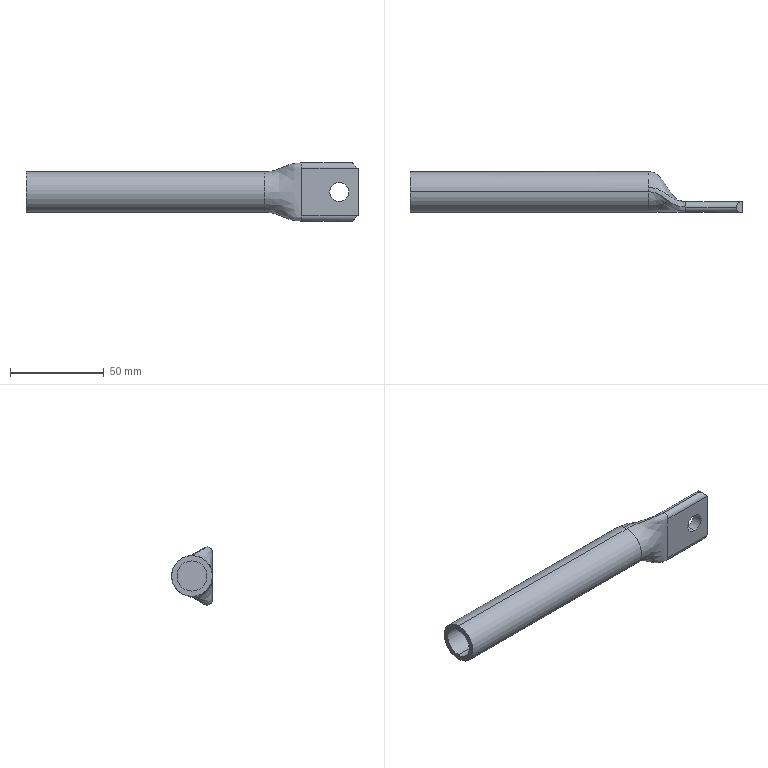Part | SolidWorks | features ICE 3, Chamfer 2, Blend 1, ExtruThin 1 | 1 solid | 28 faces | box 177 x 21.701 x 31 mm | volume 30996 mm3 | plane 15 | cylinder 10 | spline 3 | commonest cylinder face diameters 5.58 x4 10 x2 16.1 x2 21.7 x2
STEP:
#1=CARTESIAN_POINT('',(167.,-10.85,5.));
#2=VERTEX_POINT('',#1);
#3=CARTESIAN_POINT('',(167.,-10.85,-5.));
#4=VERTEX_POINT('',#3);
#5=CARTESIAN_POINT('',(167.,-10.85,0.));
#6=DIRECTION('',(0.,-1.,0.));
#7=DIRECTION('',(0.,0.,1.));
#8=AXIS2_PLACEMENT_3D('',#5,#6,#7);
#9=CIRCLE('',#8,5.);
#10=EDGE_CURVE('',#2,#4,#9,.T.);
#11=ORIENTED_EDGE('',*,*,#10,.T.);
#12=CARTESIAN_POINT('',(167.,-5.25,-5.));
#13=VERTEX_POINT('',#12);
#14=CARTESIAN_POINT('',(167.,-11.797,-5.));
#15=DIRECTION('',(0.,1.,0.));
#16=VECTOR('',#15,1000.);
#17=LINE('',#14,#16);
#18=EDGE_CURVE('',#4,#13,#17,.T.);
#19=ORIENTED_EDGE('',*,*,#18,.T.);
#20=CARTESIAN_POINT('',(167.,-5.25,5.));
#21=VERTEX_POINT('',#20);
#22=CARTESIAN_POINT('',(167.,-5.25,0.));
#23=DIRECTION('',(0.,1.,0.));
#24=DIRECTION('',(0.,0.,1.));
#25=AXIS2_PLACEMENT_3D('',#22,#23,#24);
#26=CIRCLE('',#25,5.);
#27=EDGE_CURVE('',#13,#21,#26,.T.);
#28=ORIENTED_EDGE('',*,*,#27,.T.);
#29=CARTESIAN_POINT('',(167.,-11.797,5.));
#30=DIRECTION('',(0.,1.,0.));
#31=VECTOR('',#30,1000.);
#32=LINE('',#29,#31);
#33=EDGE_CURVE('',#2,#21,#32,.T.);
#34=ORIENTED_EDGE('',*,*,#33,.F.);
#35=EDGE_LOOP('',(#11,#19,#28,#34));
#36=FACE_OUTER_BOUND('',#35,.T.);
#37=CARTESIAN_POINT('',(167.,-11.797,0.));
#38=DIRECTION('',(0.,1.,0.));
#39=DIRECTION('',(0.,0.,1.));
#40=AXIS2_PLACEMENT_3D('',#37,#38,#39);
#41=CYLINDRICAL_SURFACE('',#40,5.);
#42=ADVANCED_FACE('',(#36),#41,.F.);
#43=CARTESIAN_POINT('',(127.,0.,8.05));
#44=VERTEX_POINT('',#43);
#45=CARTESIAN_POINT('',(127.,0.,-8.05));
#46=VERTEX_POINT('',#45);
#47=CARTESIAN_POINT('',(127.,0.,0.));
#48=DIRECTION('',(1.,0.,0.));
#49=DIRECTION('',(0.,0.,-1.));
#50=AXIS2_PLACEMENT_3D('',#47,#48,#49);
#51=CIRCLE('',#50,8.05);
#52=EDGE_CURVE('',#44,#46,#51,.T.);
#53=ORIENTED_EDGE('',*,*,#52,.T.);
#54=CARTESIAN_POINT('',(0.,0.,-8.05));
#55=VERTEX_POINT('',#54);
#56=CARTESIAN_POINT('',(127.,0.,-8.05));
#57=DIRECTION('',(-1.,0.,0.));
#58=VECTOR('',#57,1000.);
#59=LINE('',#56,#58);
#60=EDGE_CURVE('',#46,#55,#59,.T.);
#61=ORIENTED_EDGE('',*,*,#60,.T.);
#62=CARTESIAN_POINT('',(0.,0.,8.05));
#63=VERTEX_POINT('',#62);
#64=CARTESIAN_POINT('',(0.,0.,0.));
#65=DIRECTION('',(1.,0.,0.));
#66=DIRECTION('',(0.,0.,-1.));
#67=AXIS2_PLACEMENT_3D('',#64,#65,#66);
#68=CIRCLE('',#67,8.05);
#69=EDGE_CURVE('',#63,#55,#68,.T.);
#70=ORIENTED_EDGE('',*,*,#69,.F.);
#71=CARTESIAN_POINT('',(127.,0.,8.05));
#72=DIRECTION('',(-1.,0.,0.));
#73=VECTOR('',#72,1000.);
#74=LINE('',#71,#73);
#75=EDGE_CURVE('',#44,#63,#74,.T.);
#76=ORIENTED_EDGE('',*,*,#75,.F.);
#77=EDGE_LOOP('',(#53,#61,#70,#76));
#78=FACE_OUTER_BOUND('',#77,.T.);
#79=CARTESIAN_POINT('',(127.,0.,0.));
#80=DIRECTION('',(-1.,0.,0.));
#81=DIRECTION('',(0.,0.,1.));
#82=AXIS2_PLACEMENT_3D('',#79,#80,#81);
#83=CYLINDRICAL_SURFACE('',#82,8.05);
#84=ADVANCED_FACE('',(#78),#83,.F.);
#85=CARTESIAN_POINT('',(127.,0.00175,-10.85));
#86=VERTEX_POINT('',#85);
#87=CARTESIAN_POINT('',(127.,2.334,10.597));
#88=VERTEX_POINT('',#87);
#89=CARTESIAN_POINT('',(127.,0.00175,-10.85));
#90=CARTESIAN_POINT('',(127.,0.3537,-10.85));
#91=CARTESIAN_POINT('',(127.,0.5767,-10.839));
#92=CARTESIAN_POINT('',(127.,0.7699,-10.825));
#93=CARTESIAN_POINT('',(127.,1.177,-10.792));
#94=CARTESIAN_POINT('',(127.,1.582,-10.736));
#95=CARTESIAN_POINT('',(127.,1.774,-10.708));
#96=CARTESIAN_POINT('',(127.,1.994,-10.671));
#97=CARTESIAN_POINT('',(127.,2.677,-10.52));
#98=CARTESIAN_POINT('',(127.,3.018,-10.431));
#99=CARTESIAN_POINT('',(127.,3.357,-10.326));
#100=CARTESIAN_POINT('',(127.,6.037,-9.379));
#101=CARTESIAN_POINT('',(127.,8.44,-7.529));
#102=CARTESIAN_POINT('',(127.,10.034,-5.273));
#103=CARTESIAN_POINT('',(127.,11.771,0.3481));
#104=CARTESIAN_POINT('',(127.,9.812,5.985));
#105=CARTESIAN_POINT('',(127.,7.737,8.454));
#106=CARTESIAN_POINT('',(127.,5.094,9.988));
#107=CARTESIAN_POINT('',(127.,2.334,10.597));
#108=B_SPLINE_CURVE_WITH_KNOTS('',5,(#89,#90,#91,#92,#93,#94,#95,#96,#97,#98,#99,#100,#101,#102,#103,#104,#105,#106,#107),.UNSPECIFIED.,.F.,.F.,(6,3,4,3,3,6),(0.,0.05525,0.1105,0.1661,0.5552,1.),.UNSPECIFIED.);
#109=EDGE_CURVE('',#86,#88,#108,.T.);
#110=ORIENTED_EDGE('',*,*,#109,.F.);
#111=CARTESIAN_POINT('',(0.,0.,-10.85));
#112=VERTEX_POINT('',#111);
#113=CARTESIAN_POINT('',(127.,0.,-10.85));
#114=DIRECTION('',(-1.,0.,0.));
#115=VECTOR('',#114,1000.);
#116=LINE('',#113,#115);
#117=EDGE_CURVE('',#86,#112,#116,.T.);
#118=ORIENTED_EDGE('',*,*,#117,.T.);
#119=CARTESIAN_POINT('',(0.,0.,10.85));
#120=VERTEX_POINT('',#119);
#121=CARTESIAN_POINT('',(0.,0.,0.));
#122=DIRECTION('',(1.,0.,0.));
#123=DIRECTION('',(0.,0.,-1.));
#124=AXIS2_PLACEMENT_3D('',#121,#122,#123);
#125=CIRCLE('',#124,10.85);
#126=EDGE_CURVE('',#112,#120,#125,.T.);
#127=ORIENTED_EDGE('',*,*,#126,.T.);
#128=CARTESIAN_POINT('',(127.,0.000003204,10.85));
#129=VERTEX_POINT('',#128);
#130=CARTESIAN_POINT('',(127.,0.,10.85));
#131=DIRECTION('',(-1.,0.,0.));
#132=VECTOR('',#131,1000.);
#133=LINE('',#130,#132);
#134=EDGE_CURVE('',#129,#120,#133,.T.);
#135=ORIENTED_EDGE('',*,*,#134,.F.);
#136=CARTESIAN_POINT('',(127.,0.,0.));
#137=DIRECTION('',(1.,0.,0.));
#138=DIRECTION('',(0.,0.,-1.));
#139=AXIS2_PLACEMENT_3D('',#136,#137,#138);
#140=CIRCLE('',#139,10.85);
#141=EDGE_CURVE('',#88,#129,#140,.T.);
#142=ORIENTED_EDGE('',*,*,#141,.F.);
#143=EDGE_LOOP('',(#110,#118,#127,#135,#142));
#144=FACE_OUTER_BOUND('',#143,.T.);
#145=CARTESIAN_POINT('',(127.,0.,0.));
#146=DIRECTION('',(-1.,0.,0.));
#147=DIRECTION('',(0.,0.,1.));
#148=AXIS2_PLACEMENT_3D('',#145,#146,#147);
#149=CYLINDRICAL_SURFACE('',#148,10.85);
#150=ADVANCED_FACE('',(#144),#149,.T.);
#151=CARTESIAN_POINT('',(177.,-8.1,12.5));
#152=VERTEX_POINT('',#151);
#153=CARTESIAN_POINT('',(177.,-8.1,-12.5));
#154=VERTEX_POINT('',#153);
#155=CARTESIAN_POINT('',(177.,-8.1,-12.5));
#156=DIRECTION('',(0.,0.,-1.));
#157=VECTOR('',#156,1000.);
#158=LINE('',#155,#157);
#159=EDGE_CURVE('',#152,#154,#158,.T.);
#160=ORIENTED_EDGE('',*,*,#159,.F.);
#161=CARTESIAN_POINT('',(177.,-10.85,12.5));
#162=VERTEX_POINT('',#161);
#163=CARTESIAN_POINT('',(177.,-8.06,12.5));
#164=DIRECTION('',(0.,-1.,0.));
#165=VECTOR('',#164,1000.);
#166=LINE('',#163,#165);
#167=EDGE_CURVE('',#152,#162,#166,.T.);
#168=ORIENTED_EDGE('',*,*,#167,.T.);
#169=CARTESIAN_POINT('',(177.,-10.85,-12.5));
#170=VERTEX_POINT('',#169);
#171=CARTESIAN_POINT('',(177.,-10.85,12.71));
#172=DIRECTION('',(0.,0.,-1.));
#173=VECTOR('',#172,1000.);
#174=LINE('',#171,#173);
#175=EDGE_CURVE('',#162,#170,#174,.T.);
#176=ORIENTED_EDGE('',*,*,#175,.T.);
#177=CARTESIAN_POINT('',(177.,-8.04,-12.5));
#178=DIRECTION('',(0.,1.,0.));
#179=VECTOR('',#178,1000.);
#180=LINE('',#177,#179);
#181=EDGE_CURVE('',#170,#154,#180,.T.);
#182=ORIENTED_EDGE('',*,*,#181,.T.);
#183=EDGE_LOOP('',(#160,#168,#176,#182));
#184=FACE_OUTER_BOUND('',#183,.T.);
#185=CARTESIAN_POINT('',(177.,-8.06,-12.71));
#186=DIRECTION('',(1.,0.,0.));
#187=DIRECTION('',(0.,0.,-1.));
#188=AXIS2_PLACEMENT_3D('',#185,#186,#187);
#189=PLANE('',#188);
#190=ADVANCED_FACE('',(#184),#189,.T.);
#191=CARTESIAN_POINT('',(0.,0.,0.));
#192=DIRECTION('',(1.,0.,0.));
#193=DIRECTION('',(0.,0.,-1.));
#194=AXIS2_PLACEMENT_3D('',#191,#192,#193);
#195=CIRCLE('',#194,10.85);
#196=EDGE_CURVE('',#120,#112,#195,.T.);
#197=ORIENTED_EDGE('',*,*,#196,.F.);
#198=ORIENTED_EDGE('',*,*,#126,.F.);
#199=EDGE_LOOP('',(#197,#198));
#200=FACE_OUTER_BOUND('',#199,.T.);
#201=ORIENTED_EDGE('',*,*,#69,.T.);
#202=CARTESIAN_POINT('',(0.,0.,0.));
#203=DIRECTION('',(1.,0.,0.));
#204=DIRECTION('',(0.,0.,-1.));
#205=AXIS2_PLACEMENT_3D('',#202,#203,#204);
#206=CIRCLE('',#205,8.05);
#207=EDGE_CURVE('',#55,#63,#206,.T.);
#208=ORIENTED_EDGE('',*,*,#207,.T.);
#209=EDGE_LOOP('',(#201,#208));
#210=FACE_BOUND('',#209,.T.);
#211=CARTESIAN_POINT('',(0.,0.,0.));
#212=DIRECTION('',(1.,0.,0.));
#213=DIRECTION('',(0.,0.,-1.));
#214=AXIS2_PLACEMENT_3D('',#211,#212,#213);
#215=PLANE('',#214);
#216=ADVANCED_FACE('',(#200,#210),#215,.F.);
#217=ORIENTED_EDGE('',*,*,#117,.F.);
#218=CARTESIAN_POINT('',(127.,0.,0.));
#219=DIRECTION('',(1.,0.,0.));
#220=DIRECTION('',(0.,0.,-1.));
#221=AXIS2_PLACEMENT_3D('',#218,#219,#220);
#222=CIRCLE('',#221,10.85);
#223=EDGE_CURVE('',#129,#86,#222,.T.);
#224=ORIENTED_EDGE('',*,*,#223,.F.);
#225=ORIENTED_EDGE('',*,*,#134,.T.);
#226=ORIENTED_EDGE('',*,*,#196,.T.);
#227=EDGE_LOOP('',(#217,#224,#225,#226));
#228=FACE_OUTER_BOUND('',#227,.T.);
#229=CARTESIAN_POINT('',(127.,0.,0.));
#230=DIRECTION('',(-1.,0.,0.));
#231=DIRECTION('',(0.,0.,1.));
#232=AXIS2_PLACEMENT_3D('',#229,#230,#231);
#233=CYLINDRICAL_SURFACE('',#232,10.85);
#234=ADVANCED_FACE('',(#228),#233,.T.);
#235=ORIENTED_EDGE('',*,*,#60,.F.);
#236=CARTESIAN_POINT('',(127.,0.,0.));
#237=DIRECTION('',(1.,0.,0.));
#238=DIRECTION('',(0.,0.,-1.));
#239=AXIS2_PLACEMENT_3D('',#236,#237,#238);
#240=CIRCLE('',#239,8.05);
#241=EDGE_CURVE('',#46,#44,#240,.T.);
#242=ORIENTED_EDGE('',*,*,#241,.T.);
#243=ORIENTED_EDGE('',*,*,#75,.T.);
#244=ORIENTED_EDGE('',*,*,#207,.F.);
#245=EDGE_LOOP('',(#235,#242,#243,#244));
#246=FACE_OUTER_BOUND('',#245,.T.);
#247=CARTESIAN_POINT('',(127.,0.,0.));
#248=DIRECTION('',(-1.,0.,0.));
#249=DIRECTION('',(0.,0.,1.));
#250=AXIS2_PLACEMENT_3D('',#247,#248,#249);
#251=CYLINDRICAL_SURFACE('',#250,8.05);
#252=ADVANCED_FACE('',(#246),#251,.F.);
#253=ORIENTED_EDGE('',*,*,#52,.F.);
#254=ORIENTED_EDGE('',*,*,#241,.F.);
#255=EDGE_LOOP('',(#253,#254));
#256=FACE_OUTER_BOUND('',#255,.T.);
#257=CARTESIAN_POINT('',(127.,0.,0.));
#258=DIRECTION('',(1.,0.,0.));
#259=DIRECTION('',(0.,0.,-1.));
#260=AXIS2_PLACEMENT_3D('',#257,#258,#259);
#261=PLANE('',#260);
#262=ADVANCED_FACE('',(#256),#261,.F.);
#263=CARTESIAN_POINT('',(147.,-5.25,12.71));
#264=VERTEX_POINT('',#263);
#265=CARTESIAN_POINT('',(147.,-5.25,12.71));
#266=CARTESIAN_POINT('',(142.97,-5.25,12.71));
#267=CARTESIAN_POINT('',(138.94,-5.25,12.71));
#268=CARTESIAN_POINT('',(135.06,2.334,10.596));
#269=CARTESIAN_POINT('',(131.03,2.334,10.596));
#270=CARTESIAN_POINT('',(127.,2.334,10.597));
#271=B_SPLINE_CURVE_WITH_KNOTS('',5,(#265,#266,#267,#268,#269,#270),.UNSPECIFIED.,.F.,.F.,(6,6),(0.,1.),.UNSPECIFIED.);
#272=EDGE_CURVE('',#264,#88,#271,.T.);
#273=ORIENTED_EDGE('',*,*,#272,.F.);
#274=CARTESIAN_POINT('',(147.,-5.25,-12.71));
#275=VERTEX_POINT('',#274);
#276=CARTESIAN_POINT('',(147.,-5.25,12.71));
#277=DIRECTION('',(0.,0.,-1.));
#278=VECTOR('',#277,1000.);
#279=LINE('',#276,#278);
#280=EDGE_CURVE('',#264,#275,#279,.T.);
#281=ORIENTED_EDGE('',*,*,#280,.T.);
#282=CARTESIAN_POINT('',(147.,-8.054,-15.5));
#283=VERTEX_POINT('',#282);
#284=CARTESIAN_POINT('',(147.,-5.25,-12.71));
#285=CARTESIAN_POINT('',(147.,-5.25,-13.038));
#286=CARTESIAN_POINT('',(147.,-5.297,-13.412));
#287=CARTESIAN_POINT('',(147.,-5.413,-13.847));
#288=CARTESIAN_POINT('',(147.,-5.978,-14.779));
#289=CARTESIAN_POINT('',(147.,-6.91,-15.339));
#290=CARTESIAN_POINT('',(147.,-7.342,-15.453));
#291=CARTESIAN_POINT('',(147.,-7.714,-15.5));
#292=CARTESIAN_POINT('',(147.,-8.054,-15.5));
#293=B_SPLINE_CURVE_WITH_KNOTS('',5,(#284,#285,#286,#287,#288,#289,#290,#291,#292),.UNSPECIFIED.,.F.,.F.,(6,3,6),(0.8895,0.9448,1.),.UNSPECIFIED.);
#294=EDGE_CURVE('',#275,#283,#293,.T.);
#295=ORIENTED_EDGE('',*,*,#294,.T.);
#296=CARTESIAN_POINT('',(147.,-8.054,-15.5));
#297=CARTESIAN_POINT('',(142.959,-8.04,-15.5));
#298=CARTESIAN_POINT('',(138.918,-8.04,-15.5));
#299=CARTESIAN_POINT('',(135.082,0.007,-10.85));
#300=CARTESIAN_POINT('',(131.041,0.007,-10.85));
#301=CARTESIAN_POINT('',(127.,0.00175,-10.85));
#302=B_SPLINE_CURVE_WITH_KNOTS('',5,(#296,#297,#298,#299,#300,#301),.UNSPECIFIED.,.F.,.F.,(6,6),(0.,1.),.UNSPECIFIED.);
#303=EDGE_CURVE('',#283,#86,#302,.T.);
#304=ORIENTED_EDGE('',*,*,#303,.T.);
#305=ORIENTED_EDGE('',*,*,#109,.T.);
#306=EDGE_LOOP('',(#273,#281,#295,#304,#305));
#307=FACE_OUTER_BOUND('',#306,.T.);
#308=CARTESIAN_POINT('',(147.,-8.04,-15.5));
#309=CARTESIAN_POINT('',(142.959,-8.04,-15.5));
#310=CARTESIAN_POINT('',(138.918,-8.04,-15.5));
#311=CARTESIAN_POINT('',(135.082,0.007,-10.85));
#312=CARTESIAN_POINT('',(131.041,0.007,-10.85));
#313=CARTESIAN_POINT('',(127.,0.007,-10.85));
#314=CARTESIAN_POINT('',(147.,-7.714,-15.5));
#315=CARTESIAN_POINT('',(142.962,-7.714,-15.5));
#316=CARTESIAN_POINT('',(138.924,-7.714,-15.5));
#317=CARTESIAN_POINT('',(135.076,0.3537,-10.85));
#318=CARTESIAN_POINT('',(131.038,0.3537,-10.85));
#319=CARTESIAN_POINT('',(127.,0.3537,-10.85));
#320=CARTESIAN_POINT('',(147.,-7.342,-15.453));
#321=CARTESIAN_POINT('',(142.965,-7.342,-15.453));
#322=CARTESIAN_POINT('',(138.929,-7.342,-15.453));
#323=CARTESIAN_POINT('',(135.071,0.5767,-10.839));
#324=CARTESIAN_POINT('',(131.035,0.5767,-10.839));
#325=CARTESIAN_POINT('',(127.,0.5767,-10.839));
#326=CARTESIAN_POINT('',(147.,-6.91,-15.339));
#327=CARTESIAN_POINT('',(142.967,-6.91,-15.339));
#328=CARTESIAN_POINT('',(138.934,-6.91,-15.339));
#329=CARTESIAN_POINT('',(135.066,0.7699,-10.825));
#330=CARTESIAN_POINT('',(131.033,0.7699,-10.825));
#331=CARTESIAN_POINT('',(127.,0.7699,-10.825));
#332=CARTESIAN_POINT('',(147.,-5.978,-14.779));
#333=CARTESIAN_POINT('',(142.97,-5.978,-14.779));
#334=CARTESIAN_POINT('',(138.939,-5.978,-14.779));
#335=CARTESIAN_POINT('',(135.061,1.177,-10.792));
#336=CARTESIAN_POINT('',(131.03,1.177,-10.792));
#337=CARTESIAN_POINT('',(127.,1.177,-10.792));
#338=CARTESIAN_POINT('',(147.,-5.413,-13.847));
#339=CARTESIAN_POINT('',(142.968,-5.413,-13.847));
#340=CARTESIAN_POINT('',(138.936,-5.413,-13.847));
#341=CARTESIAN_POINT('',(135.064,1.582,-10.736));
#342=CARTESIAN_POINT('',(131.032,1.582,-10.736));
#343=CARTESIAN_POINT('',(127.,1.582,-10.736));
#344=CARTESIAN_POINT('',(147.,-5.297,-13.412));
#345=CARTESIAN_POINT('',(142.966,-5.297,-13.412));
#346=CARTESIAN_POINT('',(138.931,-5.297,-13.412));
#347=CARTESIAN_POINT('',(135.069,1.774,-10.708));
#348=CARTESIAN_POINT('',(131.034,1.774,-10.708));
#349=CARTESIAN_POINT('',(127.,1.774,-10.708));
#350=CARTESIAN_POINT('',(147.,-5.25,-13.038));
#351=CARTESIAN_POINT('',(142.962,-5.25,-13.038));
#352=CARTESIAN_POINT('',(138.924,-5.25,-13.038));
#353=CARTESIAN_POINT('',(135.076,1.994,-10.671));
#354=CARTESIAN_POINT('',(131.038,1.994,-10.671));
#355=CARTESIAN_POINT('',(127.,1.994,-10.671));
#356=CARTESIAN_POINT('',(147.,-5.25,-12.38));
#357=CARTESIAN_POINT('',(142.95,-5.25,-12.38));
#358=CARTESIAN_POINT('',(138.9,-5.25,-12.38));
#359=CARTESIAN_POINT('',(135.1,2.677,-10.52));
#360=CARTESIAN_POINT('',(131.05,2.677,-10.52));
#361=CARTESIAN_POINT('',(127.,2.677,-10.52));
#362=CARTESIAN_POINT('',(147.,-5.25,-12.052));
#363=CARTESIAN_POINT('',(142.942,-5.25,-12.052));
#364=CARTESIAN_POINT('',(138.884,-5.25,-12.052));
#365=CARTESIAN_POINT('',(135.116,3.018,-10.431));
#366=CARTESIAN_POINT('',(131.058,3.018,-10.431));
#367=CARTESIAN_POINT('',(127.,3.018,-10.431));
#368=CARTESIAN_POINT('',(147.,-5.25,-11.724));
#369=CARTESIAN_POINT('',(142.939,-5.25,-11.724));
#370=CARTESIAN_POINT('',(138.878,-5.25,-11.724));
#371=CARTESIAN_POINT('',(135.122,3.357,-10.326));
#372=CARTESIAN_POINT('',(131.061,3.357,-10.326));
#373=CARTESIAN_POINT('',(127.,3.357,-10.326));
#374=CARTESIAN_POINT('',(147.,-5.25,-9.115));
#375=CARTESIAN_POINT('',(142.897,-5.25,-9.115));
#376=CARTESIAN_POINT('',(138.794,-5.25,-9.115));
#377=CARTESIAN_POINT('',(135.206,6.037,-9.379));
#378=CARTESIAN_POINT('',(131.103,6.037,-9.379));
#379=CARTESIAN_POINT('',(127.,6.037,-9.379));
#380=CARTESIAN_POINT('',(147.,-5.25,-6.573));
#381=CARTESIAN_POINT('',(142.868,-5.25,-6.573));
#382=CARTESIAN_POINT('',(138.736,-5.25,-6.573));
#383=CARTESIAN_POINT('',(135.264,8.44,-7.529));
#384=CARTESIAN_POINT('',(131.132,8.44,-7.529));
#385=CARTESIAN_POINT('',(127.,8.44,-7.529));
#386=CARTESIAN_POINT('',(147.,-5.25,-4.381));
#387=CARTESIAN_POINT('',(142.852,-5.25,-4.381));
#388=CARTESIAN_POINT('',(138.704,-5.25,-4.381));
#389=CARTESIAN_POINT('',(135.296,10.034,-5.273));
#390=CARTESIAN_POINT('',(131.148,10.034,-5.273));
#391=CARTESIAN_POINT('',(127.,10.034,-5.273));
#392=CARTESIAN_POINT('',(147.,-5.25,0.2909));
#393=CARTESIAN_POINT('',(142.838,-5.25,0.2909));
#394=CARTESIAN_POINT('',(138.676,-5.25,0.2909));
#395=CARTESIAN_POINT('',(135.324,11.771,0.3481));
#396=CARTESIAN_POINT('',(131.162,11.771,0.3481));
#397=CARTESIAN_POINT('',(127.,11.771,0.3481));
#398=CARTESIAN_POINT('',(147.,-5.25,4.969));
#399=CARTESIAN_POINT('',(142.865,-5.25,4.969));
#400=CARTESIAN_POINT('',(138.729,-5.25,4.969));
#401=CARTESIAN_POINT('',(135.271,9.812,5.985));
#402=CARTESIAN_POINT('',(131.135,9.812,5.985));
#403=CARTESIAN_POINT('',(127.,9.812,5.985));
#404=CARTESIAN_POINT('',(147.,-5.25,7.487));
#405=CARTESIAN_POINT('',(142.89,-5.25,7.487));
#406=CARTESIAN_POINT('',(138.779,-5.25,7.487));
#407=CARTESIAN_POINT('',(135.221,7.737,8.454));
#408=CARTESIAN_POINT('',(131.11,7.737,8.454));
#409=CARTESIAN_POINT('',(127.,7.737,8.454));
#410=CARTESIAN_POINT('',(147.,-5.25,10.055));
#411=CARTESIAN_POINT('',(142.925,-5.25,10.055));
#412=CARTESIAN_POINT('',(138.85,-5.25,10.055));
#413=CARTESIAN_POINT('',(135.15,5.094,9.988));
#414=CARTESIAN_POINT('',(131.075,5.094,9.988));
#415=CARTESIAN_POINT('',(127.,5.094,9.988));
#416=CARTESIAN_POINT('',(147.,-5.25,12.71));
#417=CARTESIAN_POINT('',(142.97,-5.25,12.71));
#418=CARTESIAN_POINT('',(138.94,-5.25,12.71));
#419=CARTESIAN_POINT('',(135.06,2.334,10.596));
#420=CARTESIAN_POINT('',(131.03,2.334,10.596));
#421=CARTESIAN_POINT('',(127.,2.334,10.596));
#422=B_SPLINE_SURFACE_WITH_KNOTS('',5,5,((#308,#309,#310,#311,#312,#313),(#314,#315,#316,#317,#318,#319),(#320,#321,#322,#323,#324,#325),(#326,#327,#328,#329,#330,#331),(#332,#333,#334,#335,#336,#337),(#338,#339,#340,#341,#342,#343),(#344,#345,#346,#347,#348,#349),(#350,#351,#352,#353,#354,#355),(#356,#357,#358,#359,#360,#361),(#362,#363,#364,#365,#366,#367),(#368,#369,#370,#371,#372,#373),(#374,#375,#376,#377,#378,#379),(#380,#381,#382,#383,#384,#385),(#386,#387,#388,#389,#390,#391),(#392,#393,#394,#395,#396,#397),(#398,#399,#400,#401,#402,#403),(#404,#405,#406,#407,#408,#409),(#410,#411,#412,#413,#414,#415),(#416,#417,#418,#419,#420,#421)),.UNSPECIFIED.,.F.,.F.,.F.,(6,3,4,3,3,6),(6,6),(0.,0.05525,0.1105,0.1661,0.5552,1.),(0.,1.),.UNSPECIFIED.);
#423=ADVANCED_FACE('',(#307),#422,.F.);
#424=ORIENTED_EDGE('',*,*,#272,.T.);
#425=ORIENTED_EDGE('',*,*,#141,.T.);
#426=CARTESIAN_POINT('',(147.,-8.046,15.5));
#427=VERTEX_POINT('',#426);
#428=CARTESIAN_POINT('',(147.,-8.046,15.5));
#429=CARTESIAN_POINT('',(142.959,-8.04,15.5));
#430=CARTESIAN_POINT('',(138.918,-8.04,15.5));
#431=CARTESIAN_POINT('',(135.082,0.007,10.85));
#432=CARTESIAN_POINT('',(131.041,0.007,10.85));
#433=CARTESIAN_POINT('',(127.,0.000003204,10.85));
#434=B_SPLINE_CURVE_WITH_KNOTS('',5,(#428,#429,#430,#431,#432,#433),.UNSPECIFIED.,.F.,.F.,(6,6),(0.,1.),.UNSPECIFIED.);
#435=EDGE_CURVE('',#427,#129,#434,.T.);
#436=ORIENTED_EDGE('',*,*,#435,.F.);
#437=CARTESIAN_POINT('',(147.,-8.04,12.71));
#438=DIRECTION('',(-1.,0.,0.));
#439=DIRECTION('',(0.,0.,1.));
#440=AXIS2_PLACEMENT_3D('',#437,#438,#439);
#441=CIRCLE('',#440,2.79);
#442=EDGE_CURVE('',#427,#264,#441,.T.);
#443=ORIENTED_EDGE('',*,*,#442,.T.);
#444=EDGE_LOOP('',(#424,#425,#436,#443));
#445=FACE_OUTER_BOUND('',#444,.T.);
#446=CARTESIAN_POINT('',(147.,-8.04,15.5));
#447=CARTESIAN_POINT('',(142.959,-8.04,15.5));
#448=CARTESIAN_POINT('',(138.918,-8.04,15.5));
#449=CARTESIAN_POINT('',(135.082,0.007,10.85));
#450=CARTESIAN_POINT('',(131.041,0.007,10.85));
#451=CARTESIAN_POINT('',(127.,0.007,10.85));
#452=CARTESIAN_POINT('',(147.,-7.116,15.5));
#453=CARTESIAN_POINT('',(142.959,-7.116,15.5));
#454=CARTESIAN_POINT('',(138.918,-7.116,15.5));
#455=CARTESIAN_POINT('',(135.082,0.4766,10.85));
#456=CARTESIAN_POINT('',(131.041,0.4766,10.85));
#457=CARTESIAN_POINT('',(127.,0.4766,10.85));
#458=CARTESIAN_POINT('',(147.,-6.279,15.125));
#459=CARTESIAN_POINT('',(142.961,-6.279,15.125));
#460=CARTESIAN_POINT('',(138.921,-6.279,15.125));
#461=CARTESIAN_POINT('',(135.079,0.9455,10.824));
#462=CARTESIAN_POINT('',(131.039,0.9455,10.824));
#463=CARTESIAN_POINT('',(127.,0.9455,10.824));
#464=CARTESIAN_POINT('',(147.,-5.625,14.471));
#465=CARTESIAN_POINT('',(142.963,-5.625,14.471));
#466=CARTESIAN_POINT('',(138.927,-5.625,14.471));
#467=CARTESIAN_POINT('',(135.073,1.412,10.773));
#468=CARTESIAN_POINT('',(131.037,1.412,10.773));
#469=CARTESIAN_POINT('',(127.,1.412,10.773));
#470=CARTESIAN_POINT('',(147.,-5.25,13.634));
#471=CARTESIAN_POINT('',(142.967,-5.25,13.634));
#472=CARTESIAN_POINT('',(138.934,-5.25,13.634));
#473=CARTESIAN_POINT('',(135.066,1.876,10.697));
#474=CARTESIAN_POINT('',(131.033,1.876,10.697));
#475=CARTESIAN_POINT('',(127.,1.876,10.697));
#476=CARTESIAN_POINT('',(147.,-5.25,12.71));
#477=CARTESIAN_POINT('',(142.97,-5.25,12.71));
#478=CARTESIAN_POINT('',(138.94,-5.25,12.71));
#479=CARTESIAN_POINT('',(135.06,2.334,10.596));
#480=CARTESIAN_POINT('',(131.03,2.334,10.596));
#481=CARTESIAN_POINT('',(127.,2.334,10.596));
#482=B_SPLINE_SURFACE_WITH_KNOTS('',5,5,((#446,#447,#448,#449,#450,#451),(#452,#453,#454,#455,#456,#457),(#458,#459,#460,#461,#462,#463),(#464,#465,#466,#467,#468,#469),(#470,#471,#472,#473,#474,#475),(#476,#477,#478,#479,#480,#481)),.UNSPECIFIED.,.F.,.F.,.F.,(6,6),(6,6),(0.,1.),(0.,1.),.UNSPECIFIED.);
#483=ADVANCED_FACE('',(#445),#482,.T.);
#484=ORIENTED_EDGE('',*,*,#303,.F.);
#485=CARTESIAN_POINT('',(147.,-10.85,-12.71));
#486=VERTEX_POINT('',#485);
#487=CARTESIAN_POINT('',(147.,-8.06,-12.71));
#488=DIRECTION('',(-1.,0.,0.));
#489=DIRECTION('',(0.,0.,1.));
#490=AXIS2_PLACEMENT_3D('',#487,#488,#489);
#491=CIRCLE('',#490,2.79);
#492=EDGE_CURVE('',#283,#486,#491,.T.);
#493=ORIENTED_EDGE('',*,*,#492,.T.);
#494=CARTESIAN_POINT('',(147.,-10.85,12.71));
#495=VERTEX_POINT('',#494);
#496=CARTESIAN_POINT('',(147.,-10.85,-12.71));
#497=DIRECTION('',(0.,0.,1.));
#498=VECTOR('',#497,1000.);
#499=LINE('',#496,#498);
#500=EDGE_CURVE('',#486,#495,#499,.T.);
#501=ORIENTED_EDGE('',*,*,#500,.T.);
#502=CARTESIAN_POINT('',(147.,-10.85,12.71));
#503=CARTESIAN_POINT('',(147.,-10.85,13.036));
#504=CARTESIAN_POINT('',(147.,-10.803,13.395));
#505=CARTESIAN_POINT('',(147.,-10.691,13.779));
#506=CARTESIAN_POINT('',(147.,-10.267,14.576));
#507=CARTESIAN_POINT('',(147.,-9.463,15.201));
#508=CARTESIAN_POINT('',(147.,-8.979,15.409));
#509=CARTESIAN_POINT('',(147.,-8.498,15.5));
#510=CARTESIAN_POINT('',(147.,-8.046,15.5));
#511=B_SPLINE_CURVE_WITH_KNOTS('',5,(#502,#503,#504,#505,#506,#507,#508,#509,#510),.UNSPECIFIED.,.F.,.F.,(6,3,6),(0.9015,0.9507,1.),.UNSPECIFIED.);
#512=EDGE_CURVE('',#495,#427,#511,.T.);
#513=ORIENTED_EDGE('',*,*,#512,.T.);
#514=ORIENTED_EDGE('',*,*,#435,.T.);
#515=ORIENTED_EDGE('',*,*,#223,.T.);
#516=EDGE_LOOP('',(#484,#493,#501,#513,#514,#515));
#517=FACE_OUTER_BOUND('',#516,.T.);
#518=CARTESIAN_POINT('',(147.,-8.06,15.5));
#519=CARTESIAN_POINT('',(142.959,-8.06,15.5));
#520=CARTESIAN_POINT('',(138.918,-8.06,15.5));
#521=CARTESIAN_POINT('',(135.082,-0.007,10.85));
#522=CARTESIAN_POINT('',(131.041,-0.007,10.85));
#523=CARTESIAN_POINT('',(127.,-0.007,10.85));
#524=CARTESIAN_POINT('',(147.,-8.498,15.5));
#525=CARTESIAN_POINT('',(142.962,-8.498,15.5));
#526=CARTESIAN_POINT('',(138.923,-8.498,15.5));
#527=CARTESIAN_POINT('',(135.077,-0.2418,10.85));
#528=CARTESIAN_POINT('',(131.038,-0.2418,10.85));
#529=CARTESIAN_POINT('',(127.,-0.2418,10.85));
#530=CARTESIAN_POINT('',(147.,-8.979,15.409));
#531=CARTESIAN_POINT('',(142.964,-8.979,15.409));
#532=CARTESIAN_POINT('',(138.928,-8.979,15.409));
#533=CARTESIAN_POINT('',(135.072,-0.4594,10.843));
#534=CARTESIAN_POINT('',(131.036,-0.4594,10.843));
#535=CARTESIAN_POINT('',(127.,-0.4594,10.843));
#536=CARTESIAN_POINT('',(147.,-9.463,15.201));
#537=CARTESIAN_POINT('',(142.966,-9.463,15.201));
#538=CARTESIAN_POINT('',(138.933,-9.463,15.201));
#539=CARTESIAN_POINT('',(135.067,-0.6681,10.832));
#540=CARTESIAN_POINT('',(131.034,-0.6681,10.832));
#541=CARTESIAN_POINT('',(127.,-0.6681,10.832));
#542=CARTESIAN_POINT('',(147.,-10.267,14.576));
#543=CARTESIAN_POINT('',(142.969,-10.267,14.576));
#544=CARTESIAN_POINT('',(138.938,-10.267,14.576));
#545=CARTESIAN_POINT('',(135.062,-1.084,10.802));
#546=CARTESIAN_POINT('',(131.031,-1.084,10.802));
#547=CARTESIAN_POINT('',(127.,-1.084,10.802));
#548=CARTESIAN_POINT('',(147.,-10.691,13.779));
#549=CARTESIAN_POINT('',(142.967,-10.691,13.779));
#550=CARTESIAN_POINT('',(138.935,-10.691,13.779));
#551=CARTESIAN_POINT('',(135.065,-1.526,10.745));
#552=CARTESIAN_POINT('',(131.033,-1.526,10.745));
#553=CARTESIAN_POINT('',(127.,-1.526,10.745));
#554=CARTESIAN_POINT('',(147.,-10.803,13.395));
#555=CARTESIAN_POINT('',(142.965,-10.803,13.395));
#556=CARTESIAN_POINT('',(138.93,-10.803,13.395));
#557=CARTESIAN_POINT('',(135.07,-1.747,10.714));
#558=CARTESIAN_POINT('',(131.035,-1.747,10.714));
#559=CARTESIAN_POINT('',(127.,-1.747,10.714));
#560=CARTESIAN_POINT('',(147.,-10.85,13.036));
#561=CARTESIAN_POINT('',(142.961,-10.85,13.036));
#562=CARTESIAN_POINT('',(138.923,-10.85,13.036));
#563=CARTESIAN_POINT('',(135.077,-1.996,10.671));
#564=CARTESIAN_POINT('',(131.039,-1.996,10.671));
#565=CARTESIAN_POINT('',(127.,-1.996,10.671));
#566=CARTESIAN_POINT('',(147.,-10.85,12.378));
#567=CARTESIAN_POINT('',(142.95,-10.85,12.378));
#568=CARTESIAN_POINT('',(138.9,-10.85,12.378));
#569=CARTESIAN_POINT('',(135.1,-2.679,10.52));
#570=CARTESIAN_POINT('',(131.05,-2.679,10.52));
#571=CARTESIAN_POINT('',(127.,-2.679,10.52));
#572=CARTESIAN_POINT('',(147.,-10.85,12.048));
#573=CARTESIAN_POINT('',(142.942,-10.85,12.048));
#574=CARTESIAN_POINT('',(138.885,-10.85,12.048));
#575=CARTESIAN_POINT('',(135.115,-3.022,10.429));
#576=CARTESIAN_POINT('',(131.058,-3.022,10.429));
#577=CARTESIAN_POINT('',(127.,-3.022,10.429));
#578=CARTESIAN_POINT('',(147.,-10.85,11.719));
#579=CARTESIAN_POINT('',(142.939,-10.85,11.719));
#580=CARTESIAN_POINT('',(138.878,-10.85,11.719));
#581=CARTESIAN_POINT('',(135.122,-3.363,10.325));
#582=CARTESIAN_POINT('',(131.061,-3.363,10.325));
#583=CARTESIAN_POINT('',(127.,-3.363,10.325));
#584=CARTESIAN_POINT('',(147.,-10.85,9.096));
#585=CARTESIAN_POINT('',(142.897,-10.85,9.096));
#586=CARTESIAN_POINT('',(138.795,-10.85,9.096));
#587=CARTESIAN_POINT('',(135.205,-6.056,9.37));
#588=CARTESIAN_POINT('',(131.103,-6.056,9.37));
#589=CARTESIAN_POINT('',(127.,-6.056,9.37));
#590=CARTESIAN_POINT('',(147.,-10.85,6.55));
#591=CARTESIAN_POINT('',(142.867,-10.85,6.55));
#592=CARTESIAN_POINT('',(138.735,-10.85,6.55));
#593=CARTESIAN_POINT('',(135.265,-8.461,7.508));
#594=CARTESIAN_POINT('',(131.133,-8.461,7.508));
#595=CARTESIAN_POINT('',(127.,-8.461,7.508));
#596=CARTESIAN_POINT('',(147.,-10.85,4.356));
#597=CARTESIAN_POINT('',(142.85,-10.85,4.356));
#598=CARTESIAN_POINT('',(138.699,-10.85,4.356));
#599=CARTESIAN_POINT('',(135.301,-10.047,5.246));
#600=CARTESIAN_POINT('',(131.15,-10.047,5.246));
#601=CARTESIAN_POINT('',(127.,-10.047,5.246));
#602=CARTESIAN_POINT('',(147.,-10.85,-0.3115));
#603=CARTESIAN_POINT('',(142.831,-10.85,-0.3115));
#604=CARTESIAN_POINT('',(138.661,-10.85,-0.3115));
#605=CARTESIAN_POINT('',(135.339,-11.768,-0.3742));
#606=CARTESIAN_POINT('',(131.169,-11.768,-0.3742));
#607=CARTESIAN_POINT('',(127.,-11.768,-0.3742));
#608=CARTESIAN_POINT('',(147.,-10.85,-4.979));
#609=CARTESIAN_POINT('',(142.852,-10.85,-4.979));
#610=CARTESIAN_POINT('',(138.704,-10.85,-4.979));
#611=CARTESIAN_POINT('',(135.296,-9.802,-5.994));
#612=CARTESIAN_POINT('',(131.148,-9.802,-5.994));
#613=CARTESIAN_POINT('',(127.,-9.802,-5.994));
#614=CARTESIAN_POINT('',(147.,-10.85,-7.491));
#615=CARTESIAN_POINT('',(142.875,-10.85,-7.491));
#616=CARTESIAN_POINT('',(138.75,-10.85,-7.491));
#617=CARTESIAN_POINT('',(135.25,-7.734,-8.455));
#618=CARTESIAN_POINT('',(131.125,-7.734,-8.455));
#619=CARTESIAN_POINT('',(127.,-7.734,-8.455));
#620=CARTESIAN_POINT('',(147.,-10.85,-10.056));
#621=CARTESIAN_POINT('',(142.91,-10.85,-10.056));
#622=CARTESIAN_POINT('',(138.819,-10.85,-10.056));
#623=CARTESIAN_POINT('',(135.181,-5.094,-9.988));
#624=CARTESIAN_POINT('',(131.09,-5.094,-9.988));
#625=CARTESIAN_POINT('',(127.,-5.094,-9.988));
#626=CARTESIAN_POINT('',(147.,-10.85,-13.036));
#627=CARTESIAN_POINT('',(142.961,-10.85,-13.036));
#628=CARTESIAN_POINT('',(138.923,-10.85,-13.036));
#629=CARTESIAN_POINT('',(135.077,-1.995,-10.671));
#630=CARTESIAN_POINT('',(131.039,-1.995,-10.671));
#631=CARTESIAN_POINT('',(127.,-1.995,-10.671));
#632=CARTESIAN_POINT('',(147.,-10.803,-13.395));
#633=CARTESIAN_POINT('',(142.967,-10.803,-13.395));
#634=CARTESIAN_POINT('',(138.934,-10.803,-13.395));
#635=CARTESIAN_POINT('',(135.066,-1.746,-10.714));
#636=CARTESIAN_POINT('',(131.033,-1.746,-10.714));
#637=CARTESIAN_POINT('',(127.,-1.746,-10.714));
#638=CARTESIAN_POINT('',(147.,-10.691,-13.779));
#639=CARTESIAN_POINT('',(142.967,-10.691,-13.779));
#640=CARTESIAN_POINT('',(138.935,-10.691,-13.779));
#641=CARTESIAN_POINT('',(135.065,-1.524,-10.746));
#642=CARTESIAN_POINT('',(131.033,-1.524,-10.746));
#643=CARTESIAN_POINT('',(127.,-1.524,-10.746));
#644=CARTESIAN_POINT('',(147.,-10.267,-14.576));
#645=CARTESIAN_POINT('',(142.969,-10.267,-14.576));
#646=CARTESIAN_POINT('',(138.938,-10.267,-14.576));
#647=CARTESIAN_POINT('',(135.062,-1.08,-10.802));
#648=CARTESIAN_POINT('',(131.031,-1.08,-10.802));
#649=CARTESIAN_POINT('',(127.,-1.08,-10.802));
#650=CARTESIAN_POINT('',(147.,-9.463,-15.201));
#651=CARTESIAN_POINT('',(142.966,-9.463,-15.201));
#652=CARTESIAN_POINT('',(138.932,-9.463,-15.201));
#653=CARTESIAN_POINT('',(135.068,-0.6627,-10.833));
#654=CARTESIAN_POINT('',(131.034,-0.6627,-10.833));
#655=CARTESIAN_POINT('',(127.,-0.6627,-10.833));
#656=CARTESIAN_POINT('',(147.,-8.979,-15.409));
#657=CARTESIAN_POINT('',(142.964,-8.979,-15.409));
#658=CARTESIAN_POINT('',(138.928,-8.979,-15.409));
#659=CARTESIAN_POINT('',(135.072,-0.4532,-10.844));
#660=CARTESIAN_POINT('',(131.036,-0.4532,-10.844));
#661=CARTESIAN_POINT('',(127.,-0.4532,-10.844));
#662=CARTESIAN_POINT('',(147.,-8.498,-15.5));
#663=CARTESIAN_POINT('',(142.962,-8.498,-15.5));
#664=CARTESIAN_POINT('',(138.923,-8.498,-15.5));
#665=CARTESIAN_POINT('',(135.077,-0.235,-10.85));
#666=CARTESIAN_POINT('',(131.038,-0.235,-10.85));
#667=CARTESIAN_POINT('',(127.,-0.235,-10.85));
#668=CARTESIAN_POINT('',(147.,-8.06,-15.5));
#669=CARTESIAN_POINT('',(142.959,-8.06,-15.5));
#670=CARTESIAN_POINT('',(138.918,-8.06,-15.5));
#671=CARTESIAN_POINT('',(135.082,0.,-10.85));
#672=CARTESIAN_POINT('',(131.041,0.,-10.85));
#673=CARTESIAN_POINT('',(127.,0.,-10.85));
#674=B_SPLINE_SURFACE_WITH_KNOTS('',5,5,((#518,#519,#520,#521,#522,#523),(#524,#525,#526,#527,#528,#529),(#530,#531,#532,#533,#534,#535),(#536,#537,#538,#539,#540,#541),(#542,#543,#544,#545,#546,#547),(#548,#549,#550,#551,#552,#553),(#554,#555,#556,#557,#558,#559),(#560,#561,#562,#563,#564,#565),(#566,#567,#568,#569,#570,#571),(#572,#573,#574,#575,#576,#577),(#578,#579,#580,#581,#582,#583),(#584,#585,#586,#587,#588,#589),(#590,#591,#592,#593,#594,#595),(#596,#597,#598,#599,#600,#601),(#602,#603,#604,#605,#606,#607),(#608,#609,#610,#611,#612,#613),(#614,#615,#616,#617,#618,#619),(#620,#621,#622,#623,#624,#625),(#626,#627,#628,#629,#630,#631),(#632,#633,#634,#635,#636,#637),(#638,#639,#640,#641,#642,#643),(#644,#645,#646,#647,#648,#649),(#650,#651,#652,#653,#654,#655),(#656,#657,#658,#659,#660,#661),(#662,#663,#664,#665,#666,#667),(#668,#669,#670,#671,#672,#673)),.UNSPECIFIED.,.F.,.F.,.F.,(6,3,4,3,3,4,3,6),(6,6),(0.,0.04926,0.09852,0.1487,0.4999,0.9014,0.9507,1.),(0.,1.),.UNSPECIFIED.);
#675=ADVANCED_FACE('',(#517),#674,.F.);
#676=CARTESIAN_POINT('',(174.,-8.06,-15.5));
#677=VERTEX_POINT('',#676);
#678=CARTESIAN_POINT('',(177.,-8.06,-15.5));
#679=DIRECTION('',(-1.,0.,0.));
#680=VECTOR('',#679,1000.);
#681=LINE('',#678,#680);
#682=EDGE_CURVE('',#677,#283,#681,.T.);
#683=ORIENTED_EDGE('',*,*,#682,.F.);
#684=CARTESIAN_POINT('',(176.79,-10.85,-12.71));
#685=VERTEX_POINT('',#684);
#686=CARTESIAN_POINT('',(174.,-8.06,-15.5));
#687=CARTESIAN_POINT('',(174.,-9.694,-15.5));
#688=CARTESIAN_POINT('',(175.156,-10.85,-14.344));
#689=CARTESIAN_POINT('',(176.79,-10.85,-12.71));
#690=(BOUNDED_CURVE()B_SPLINE_CURVE(3,(#686,#687,#688,#689),.UNSPECIFIED.,.F.,.T.)B_SPLINE_CURVE_WITH_KNOTS((4,4),(0.,1.571),.UNSPECIFIED.)CURVE()GEOMETRIC_REPRESENTATION_ITEM()RATIONAL_B_SPLINE_CURVE((1.,0.8047,0.8047,1.))REPRESENTATION_ITEM(''));
#691=EDGE_CURVE('',#677,#685,#690,.T.);
#692=ORIENTED_EDGE('',*,*,#691,.T.);
#693=CARTESIAN_POINT('',(177.,-10.85,-12.71));
#694=DIRECTION('',(-1.,0.,0.));
#695=VECTOR('',#694,1000.);
#696=LINE('',#693,#695);
#697=EDGE_CURVE('',#685,#486,#696,.T.);
#698=ORIENTED_EDGE('',*,*,#697,.T.);
#699=ORIENTED_EDGE('',*,*,#492,.F.);
#700=EDGE_LOOP('',(#683,#692,#698,#699));
#701=FACE_OUTER_BOUND('',#700,.T.);
#702=CARTESIAN_POINT('',(177.,-8.06,-12.71));
#703=DIRECTION('',(-1.,0.,0.));
#704=DIRECTION('',(0.,0.,1.));
#705=AXIS2_PLACEMENT_3D('',#702,#703,#704);
#706=CYLINDRICAL_SURFACE('',#705,2.79);
#707=ADVANCED_FACE('',(#701),#706,.T.);
#708=CARTESIAN_POINT('',(174.,-8.04,-15.5));
#709=VERTEX_POINT('',#708);
#710=CARTESIAN_POINT('',(177.,-8.04,-15.5));
#711=DIRECTION('',(-1.,0.,0.));
#712=VECTOR('',#711,1000.);
#713=LINE('',#710,#712);
#714=EDGE_CURVE('',#709,#283,#713,.T.);
#715=ORIENTED_EDGE('',*,*,#714,.F.);
#716=CARTESIAN_POINT('',(174.,-8.06,-15.5));
#717=DIRECTION('',(0.,-1.,0.));
#718=VECTOR('',#717,1000.);
#719=LINE('',#716,#718);
#720=EDGE_CURVE('',#709,#677,#719,.T.);
#721=ORIENTED_EDGE('',*,*,#720,.T.);
#722=ORIENTED_EDGE('',*,*,#682,.T.);
#723=EDGE_LOOP('',(#715,#721,#722));
#724=FACE_OUTER_BOUND('',#723,.T.);
#725=CARTESIAN_POINT('',(177.,-8.04,-15.5));
#726=DIRECTION('',(0.,0.,1.));
#727=DIRECTION('',(1.,0.,0.));
#728=AXIS2_PLACEMENT_3D('',#725,#726,#727);
#729=PLANE('',#728);
#730=ADVANCED_FACE('',(#724),#729,.F.);
#731=CARTESIAN_POINT('',(176.79,-5.25,-12.71));
#732=VERTEX_POINT('',#731);
#733=CARTESIAN_POINT('',(177.,-5.25,-12.71));
#734=DIRECTION('',(-1.,0.,0.));
#735=VECTOR('',#734,1000.);
#736=LINE('',#733,#735);
#737=EDGE_CURVE('',#732,#275,#736,.T.);
#738=ORIENTED_EDGE('',*,*,#737,.F.);
#739=CARTESIAN_POINT('',(176.79,-5.25,-12.71));
#740=CARTESIAN_POINT('',(175.156,-5.25,-14.344));
#741=CARTESIAN_POINT('',(174.,-6.406,-15.5));
#742=CARTESIAN_POINT('',(174.,-8.04,-15.5));
#743=(BOUNDED_CURVE()B_SPLINE_CURVE(3,(#739,#740,#741,#742),.UNSPECIFIED.,.F.,.T.)B_SPLINE_CURVE_WITH_KNOTS((4,4),(4.712,6.283),.UNSPECIFIED.)CURVE()GEOMETRIC_REPRESENTATION_ITEM()RATIONAL_B_SPLINE_CURVE((1.,0.8047,0.8047,1.))REPRESENTATION_ITEM(''));
#744=EDGE_CURVE('',#732,#709,#743,.T.);
#745=ORIENTED_EDGE('',*,*,#744,.T.);
#746=ORIENTED_EDGE('',*,*,#714,.T.);
#747=ORIENTED_EDGE('',*,*,#294,.F.);
#748=EDGE_LOOP('',(#738,#745,#746,#747));
#749=FACE_OUTER_BOUND('',#748,.T.);
#750=CARTESIAN_POINT('',(177.,-8.04,-12.71));
#751=DIRECTION('',(-1.,0.,0.));
#752=DIRECTION('',(0.,0.,1.));
#753=AXIS2_PLACEMENT_3D('',#750,#751,#752);
#754=CYLINDRICAL_SURFACE('',#753,2.79);
#755=ADVANCED_FACE('',(#749),#754,.T.);
#756=CARTESIAN_POINT('',(167.,-5.25,0.));
#757=DIRECTION('',(0.,1.,0.));
#758=DIRECTION('',(0.,0.,1.));
#759=AXIS2_PLACEMENT_3D('',#756,#757,#758);
#760=CIRCLE('',#759,5.);
#761=EDGE_CURVE('',#21,#13,#760,.T.);
#762=ORIENTED_EDGE('',*,*,#761,.F.);
#763=ORIENTED_EDGE('',*,*,#27,.F.);
#764=EDGE_LOOP('',(#762,#763));
#765=FACE_BOUND('',#764,.T.);
#766=CARTESIAN_POINT('',(176.79,-5.25,12.71));
#767=VERTEX_POINT('',#766);
#768=CARTESIAN_POINT('',(177.,-5.25,12.71));
#769=DIRECTION('',(-1.,0.,0.));
#770=VECTOR('',#769,1000.);
#771=LINE('',#768,#770);
#772=EDGE_CURVE('',#767,#264,#771,.T.);
#773=ORIENTED_EDGE('',*,*,#772,.F.);
#774=CARTESIAN_POINT('',(177.,-5.25,12.5));
#775=VERTEX_POINT('',#774);
#776=CARTESIAN_POINT('',(177.,-5.25,12.5));
#777=DIRECTION('',(0.7071,0.,-0.7071));
#778=VECTOR('',#777,1000.);
#779=LINE('',#776,#778);
#780=EDGE_CURVE('',#767,#775,#779,.T.);
#781=ORIENTED_EDGE('',*,*,#780,.T.);
#782=CARTESIAN_POINT('',(177.,-5.25,-12.5));
#783=VERTEX_POINT('',#782);
#784=CARTESIAN_POINT('',(177.,-5.25,12.71));
#785=DIRECTION('',(0.,0.,1.));
#786=VECTOR('',#785,1000.);
#787=LINE('',#784,#786);
#788=EDGE_CURVE('',#783,#775,#787,.T.);
#789=ORIENTED_EDGE('',*,*,#788,.F.);
#790=CARTESIAN_POINT('',(177.,-5.25,-12.5));
#791=DIRECTION('',(-0.7071,0.,-0.7071));
#792=VECTOR('',#791,1000.);
#793=LINE('',#790,#792);
#794=EDGE_CURVE('',#783,#732,#793,.T.);
#795=ORIENTED_EDGE('',*,*,#794,.T.);
#796=ORIENTED_EDGE('',*,*,#737,.T.);
#797=ORIENTED_EDGE('',*,*,#280,.F.);
#798=EDGE_LOOP('',(#773,#781,#789,#795,#796,#797));
#799=FACE_OUTER_BOUND('',#798,.T.);
#800=CARTESIAN_POINT('',(177.,-5.25,12.71));
#801=DIRECTION('',(0.,-1.,0.));
#802=DIRECTION('',(0.,0.,-1.));
#803=AXIS2_PLACEMENT_3D('',#800,#801,#802);
#804=PLANE('',#803);
#805=ADVANCED_FACE('',(#765,#799),#804,.F.);
#806=CARTESIAN_POINT('',(174.,-8.04,15.5));
#807=VERTEX_POINT('',#806);
#808=CARTESIAN_POINT('',(177.,-8.04,15.5));
#809=DIRECTION('',(-1.,0.,0.));
#810=VECTOR('',#809,1000.);
#811=LINE('',#808,#810);
#812=EDGE_CURVE('',#807,#427,#811,.T.);
#813=ORIENTED_EDGE('',*,*,#812,.F.);
#814=CARTESIAN_POINT('',(174.,-8.04,15.5));
#815=CARTESIAN_POINT('',(174.,-6.406,15.5));
#816=CARTESIAN_POINT('',(175.156,-5.25,14.344));
#817=CARTESIAN_POINT('',(176.79,-5.25,12.71));
#818=(BOUNDED_CURVE()B_SPLINE_CURVE(3,(#814,#815,#816,#817),.UNSPECIFIED.,.F.,.T.)B_SPLINE_CURVE_WITH_KNOTS((4,4),(0.,1.571),.UNSPECIFIED.)CURVE()GEOMETRIC_REPRESENTATION_ITEM()RATIONAL_B_SPLINE_CURVE((1.,0.8047,0.8047,1.))REPRESENTATION_ITEM(''));
#819=EDGE_CURVE('',#807,#767,#818,.T.);
#820=ORIENTED_EDGE('',*,*,#819,.T.);
#821=ORIENTED_EDGE('',*,*,#772,.T.);
#822=ORIENTED_EDGE('',*,*,#442,.F.);
#823=EDGE_LOOP('',(#813,#820,#821,#822));
#824=FACE_OUTER_BOUND('',#823,.T.);
#825=CARTESIAN_POINT('',(177.,-8.04,12.71));
#826=DIRECTION('',(-1.,0.,0.));
#827=DIRECTION('',(0.,0.,1.));
#828=AXIS2_PLACEMENT_3D('',#825,#826,#827);
#829=CYLINDRICAL_SURFACE('',#828,2.79);
#830=ADVANCED_FACE('',(#824),#829,.T.);
#831=CARTESIAN_POINT('',(174.,-8.06,15.5));
#832=VERTEX_POINT('',#831);
#833=CARTESIAN_POINT('',(177.,-8.06,15.5));
#834=DIRECTION('',(-1.,0.,0.));
#835=VECTOR('',#834,1000.);
#836=LINE('',#833,#835);
#837=EDGE_CURVE('',#832,#427,#836,.T.);
#838=ORIENTED_EDGE('',*,*,#837,.F.);
#839=CARTESIAN_POINT('',(174.,-8.04,15.5));
#840=DIRECTION('',(0.,1.,0.));
#841=VECTOR('',#840,1000.);
#842=LINE('',#839,#841);
#843=EDGE_CURVE('',#832,#807,#842,.T.);
#844=ORIENTED_EDGE('',*,*,#843,.T.);
#845=ORIENTED_EDGE('',*,*,#812,.T.);
#846=EDGE_LOOP('',(#838,#844,#845));
#847=FACE_OUTER_BOUND('',#846,.T.);
#848=CARTESIAN_POINT('',(177.,-8.04,15.5));
#849=DIRECTION('',(0.,0.,-1.));
#850=DIRECTION('',(0.,1.,0.));
#851=AXIS2_PLACEMENT_3D('',#848,#849,#850);
#852=PLANE('',#851);
#853=ADVANCED_FACE('',(#847),#852,.F.);
#854=CARTESIAN_POINT('',(176.79,-10.85,12.71));
#855=VERTEX_POINT('',#854);
#856=CARTESIAN_POINT('',(177.,-10.85,12.71));
#857=DIRECTION('',(-1.,0.,0.));
#858=VECTOR('',#857,1000.);
#859=LINE('',#856,#858);
#860=EDGE_CURVE('',#855,#495,#859,.T.);
#861=ORIENTED_EDGE('',*,*,#860,.F.);
#862=CARTESIAN_POINT('',(176.79,-10.85,12.71));
#863=CARTESIAN_POINT('',(175.156,-10.85,14.344));
#864=CARTESIAN_POINT('',(174.,-9.694,15.5));
#865=CARTESIAN_POINT('',(174.,-8.06,15.5));
#866=(BOUNDED_CURVE()B_SPLINE_CURVE(3,(#862,#863,#864,#865),.UNSPECIFIED.,.F.,.F.)B_SPLINE_CURVE_WITH_KNOTS((4,4),(4.712,6.283),.UNSPECIFIED.)CURVE()GEOMETRIC_REPRESENTATION_ITEM()RATIONAL_B_SPLINE_CURVE((1.,0.8047,0.8047,1.))REPRESENTATION_ITEM(''));
#867=EDGE_CURVE('',#855,#832,#866,.T.);
#868=ORIENTED_EDGE('',*,*,#867,.T.);
#869=ORIENTED_EDGE('',*,*,#837,.T.);
#870=ORIENTED_EDGE('',*,*,#512,.F.);
#871=EDGE_LOOP('',(#861,#868,#869,#870));
#872=FACE_OUTER_BOUND('',#871,.T.);
#873=CARTESIAN_POINT('',(177.,-8.06,12.71));
#874=DIRECTION('',(-1.,0.,0.));
#875=DIRECTION('',(0.,0.,1.));
#876=AXIS2_PLACEMENT_3D('',#873,#874,#875);
#877=CYLINDRICAL_SURFACE('',#876,2.79);
#878=ADVANCED_FACE('',(#872),#877,.T.);
#879=ORIENTED_EDGE('',*,*,#10,.F.);
#880=CARTESIAN_POINT('',(167.,-10.85,0.));
#881=DIRECTION('',(0.,-1.,0.));
#882=DIRECTION('',(0.,0.,1.));
#883=AXIS2_PLACEMENT_3D('',#880,#881,#882);
#884=CIRCLE('',#883,5.);
#885=EDGE_CURVE('',#4,#2,#884,.T.);
#886=ORIENTED_EDGE('',*,*,#885,.F.);
#887=EDGE_LOOP('',(#879,#886));
#888=FACE_BOUND('',#887,.T.);
#889=ORIENTED_EDGE('',*,*,#175,.F.);
#890=CARTESIAN_POINT('',(177.,-10.85,12.5));
#891=DIRECTION('',(-0.7071,0.,0.7071));
#892=VECTOR('',#891,1000.);
#893=LINE('',#890,#892);
#894=EDGE_CURVE('',#162,#855,#893,.T.);
#895=ORIENTED_EDGE('',*,*,#894,.T.);
#896=ORIENTED_EDGE('',*,*,#860,.T.);
#897=ORIENTED_EDGE('',*,*,#500,.F.);
#898=ORIENTED_EDGE('',*,*,#697,.F.);
#899=CARTESIAN_POINT('',(177.,-10.85,-12.5));
#900=DIRECTION('',(0.7071,0.,0.7071));
#901=VECTOR('',#900,1000.);
#902=LINE('',#899,#901);
#903=EDGE_CURVE('',#685,#170,#902,.T.);
#904=ORIENTED_EDGE('',*,*,#903,.T.);
#905=EDGE_LOOP('',(#889,#895,#896,#897,#898,#904));
#906=FACE_OUTER_BOUND('',#905,.T.);
#907=CARTESIAN_POINT('',(177.,-10.85,12.71));
#908=DIRECTION('',(0.,1.,0.));
#909=DIRECTION('',(0.,0.,1.));
#910=AXIS2_PLACEMENT_3D('',#907,#908,#909);
#911=PLANE('',#910);
#912=ADVANCED_FACE('',(#888,#906),#911,.F.);
#913=CARTESIAN_POINT('',(177.,-8.,-12.5));
#914=VERTEX_POINT('',#913);
#915=CARTESIAN_POINT('',(177.,-8.,12.5));
#916=VERTEX_POINT('',#915);
#917=CARTESIAN_POINT('',(177.,-8.,-12.5));
#918=DIRECTION('',(0.,0.,1.));
#919=VECTOR('',#918,1000.);
#920=LINE('',#917,#919);
#921=EDGE_CURVE('',#914,#916,#920,.T.);
#922=ORIENTED_EDGE('',*,*,#921,.F.);
#923=CARTESIAN_POINT('',(177.,-8.04,-12.5));
#924=DIRECTION('',(0.,1.,0.));
#925=VECTOR('',#924,1000.);
#926=LINE('',#923,#925);
#927=EDGE_CURVE('',#914,#783,#926,.T.);
#928=ORIENTED_EDGE('',*,*,#927,.T.);
#929=ORIENTED_EDGE('',*,*,#788,.T.);
#930=CARTESIAN_POINT('',(177.,-8.06,12.5));
#931=DIRECTION('',(0.,-1.,0.));
#932=VECTOR('',#931,1000.);
#933=LINE('',#930,#932);
#934=EDGE_CURVE('',#775,#916,#933,.T.);
#935=ORIENTED_EDGE('',*,*,#934,.T.);
#936=EDGE_LOOP('',(#922,#928,#929,#935));
#937=FACE_OUTER_BOUND('',#936,.T.);
#938=CARTESIAN_POINT('',(177.,-8.06,-12.71));
#939=DIRECTION('',(1.,0.,0.));
#940=DIRECTION('',(0.,0.,-1.));
#941=AXIS2_PLACEMENT_3D('',#938,#939,#940);
#942=PLANE('',#941);
#943=ADVANCED_FACE('',(#937),#942,.T.);
#944=ORIENTED_EDGE('',*,*,#691,.F.);
#945=ORIENTED_EDGE('',*,*,#720,.F.);
#946=ORIENTED_EDGE('',*,*,#744,.F.);
#947=ORIENTED_EDGE('',*,*,#794,.F.);
#948=ORIENTED_EDGE('',*,*,#927,.F.);
#949=CARTESIAN_POINT('',(177.,-8.,-12.5));
#950=DIRECTION('',(0.,1.,0.));
#951=VECTOR('',#950,1000.);
#952=LINE('',#949,#951);
#953=EDGE_CURVE('',#154,#914,#952,.T.);
#954=ORIENTED_EDGE('',*,*,#953,.F.);
#955=ORIENTED_EDGE('',*,*,#181,.F.);
#956=ORIENTED_EDGE('',*,*,#903,.F.);
#957=EDGE_LOOP('',(#944,#945,#946,#947,#948,#954,#955,#956));
#958=FACE_OUTER_BOUND('',#957,.T.);
#959=CARTESIAN_POINT('',(177.,-8.06,-12.5));
#960=DIRECTION('',(0.7071,0.,-0.7071));
#961=DIRECTION('',(0.,-1.,0.));
#962=AXIS2_PLACEMENT_3D('',#959,#960,#961);
#963=PLANE('',#962);
#964=ADVANCED_FACE('',(#958),#963,.T.);
#965=ORIENTED_EDGE('',*,*,#819,.F.);
#966=ORIENTED_EDGE('',*,*,#843,.F.);
#967=ORIENTED_EDGE('',*,*,#867,.F.);
#968=ORIENTED_EDGE('',*,*,#894,.F.);
#969=ORIENTED_EDGE('',*,*,#167,.F.);
#970=CARTESIAN_POINT('',(177.,-8.,12.5));
#971=DIRECTION('',(0.,-1.,0.));
#972=VECTOR('',#971,1000.);
#973=LINE('',#970,#972);
#974=EDGE_CURVE('',#916,#152,#973,.T.);
#975=ORIENTED_EDGE('',*,*,#974,.F.);
#976=ORIENTED_EDGE('',*,*,#934,.F.);
#977=ORIENTED_EDGE('',*,*,#780,.F.);
#978=EDGE_LOOP('',(#965,#966,#967,#968,#969,#975,#976,#977));
#979=FACE_OUTER_BOUND('',#978,.T.);
#980=CARTESIAN_POINT('',(177.,-8.06,12.5));
#981=DIRECTION('',(0.7071,0.,0.7071));
#982=DIRECTION('',(0.,1.,0.));
#983=AXIS2_PLACEMENT_3D('',#980,#981,#982);
#984=PLANE('',#983);
#985=ADVANCED_FACE('',(#979),#984,.T.);
#986=ORIENTED_EDGE('',*,*,#18,.F.);
#987=ORIENTED_EDGE('',*,*,#885,.T.);
#988=ORIENTED_EDGE('',*,*,#33,.T.);
#989=ORIENTED_EDGE('',*,*,#761,.T.);
#990=EDGE_LOOP('',(#986,#987,#988,#989));
#991=FACE_OUTER_BOUND('',#990,.T.);
#992=CARTESIAN_POINT('',(167.,-11.797,0.));
#993=DIRECTION('',(0.,1.,0.));
#994=DIRECTION('',(0.,0.,1.));
#995=AXIS2_PLACEMENT_3D('',#992,#993,#994);
#996=CYLINDRICAL_SURFACE('',#995,5.);
#997=ADVANCED_FACE('',(#991),#996,.F.);
#998=ORIENTED_EDGE('',*,*,#953,.T.);
#999=CARTESIAN_POINT('',(176.9,-8.,-12.5));
#1000=VERTEX_POINT('',#999);
#1001=CARTESIAN_POINT('',(176.9,-8.,-12.5));
#1002=DIRECTION('',(1.,0.,0.));
#1003=VECTOR('',#1002,1000.);
#1004=LINE('',#1001,#1003);
#1005=EDGE_CURVE('',#1000,#914,#1004,.T.);
#1006=ORIENTED_EDGE('',*,*,#1005,.F.);
#1007=CARTESIAN_POINT('',(176.9,-8.1,-12.5));
#1008=VERTEX_POINT('',#1007);
#1009=CARTESIAN_POINT('',(176.9,-8.,-12.5));
#1010=DIRECTION('',(0.,1.,0.));
#1011=VECTOR('',#1010,1000.);
#1012=LINE('',#1009,#1011);
#1013=EDGE_CURVE('',#1008,#1000,#1012,.T.);
#1014=ORIENTED_EDGE('',*,*,#1013,.F.);
#1015=CARTESIAN_POINT('',(176.9,-8.1,-12.5));
#1016=DIRECTION('',(1.,0.,0.));
#1017=VECTOR('',#1016,1000.);
#1018=LINE('',#1015,#1017);
#1019=EDGE_CURVE('',#1008,#154,#1018,.T.);
#1020=ORIENTED_EDGE('',*,*,#1019,.T.);
#1021=EDGE_LOOP('',(#998,#1006,#1014,#1020));
#1022=FACE_OUTER_BOUND('',#1021,.T.);
#1023=CARTESIAN_POINT('',(176.9,-8.,-12.5));
#1024=DIRECTION('',(0.,0.,-1.));
#1025=DIRECTION('',(-1.,0.,0.));
#1026=AXIS2_PLACEMENT_3D('',#1023,#1024,#1025);
#1027=PLANE('',#1026);
#1028=ADVANCED_FACE('',(#1022),#1027,.F.);
#1029=ORIENTED_EDGE('',*,*,#159,.T.);
#1030=ORIENTED_EDGE('',*,*,#1019,.F.);
#1031=CARTESIAN_POINT('',(176.9,-8.1,12.5));
#1032=VERTEX_POINT('',#1031);
#1033=CARTESIAN_POINT('',(176.9,-8.1,-12.5));
#1034=DIRECTION('',(0.,0.,-1.));
#1035=VECTOR('',#1034,1000.);
#1036=LINE('',#1033,#1035);
#1037=EDGE_CURVE('',#1032,#1008,#1036,.T.);
#1038=ORIENTED_EDGE('',*,*,#1037,.F.);
#1039=CARTESIAN_POINT('',(176.9,-8.1,12.5));
#1040=DIRECTION('',(1.,0.,0.));
#1041=VECTOR('',#1040,1000.);
#1042=LINE('',#1039,#1041);
#1043=EDGE_CURVE('',#1032,#152,#1042,.T.);
#1044=ORIENTED_EDGE('',*,*,#1043,.T.);
#1045=EDGE_LOOP('',(#1029,#1030,#1038,#1044));
#1046=FACE_OUTER_BOUND('',#1045,.T.);
#1047=CARTESIAN_POINT('',(176.9,-8.1,-12.5));
#1048=DIRECTION('',(0.,-1.,0.));
#1049=DIRECTION('',(0.,0.,-1.));
#1050=AXIS2_PLACEMENT_3D('',#1047,#1048,#1049);
#1051=PLANE('',#1050);
#1052=ADVANCED_FACE('',(#1046),#1051,.F.);
#1053=ORIENTED_EDGE('',*,*,#974,.T.);
#1054=ORIENTED_EDGE('',*,*,#1043,.F.);
#1055=CARTESIAN_POINT('',(176.9,-8.,12.5));
#1056=VERTEX_POINT('',#1055);
#1057=CARTESIAN_POINT('',(176.9,-8.,12.5));
#1058=DIRECTION('',(0.,-1.,0.));
#1059=VECTOR('',#1058,1000.);
#1060=LINE('',#1057,#1059);
#1061=EDGE_CURVE('',#1056,#1032,#1060,.T.);
#1062=ORIENTED_EDGE('',*,*,#1061,.F.);
#1063=CARTESIAN_POINT('',(176.9,-8.,12.5));
#1064=DIRECTION('',(1.,0.,0.));
#1065=VECTOR('',#1064,1000.);
#1066=LINE('',#1063,#1065);
#1067=EDGE_CURVE('',#1056,#916,#1066,.T.);
#1068=ORIENTED_EDGE('',*,*,#1067,.T.);
#1069=EDGE_LOOP('',(#1053,#1054,#1062,#1068));
#1070=FACE_OUTER_BOUND('',#1069,.T.);
#1071=CARTESIAN_POINT('',(176.9,-8.,12.5));
#1072=DIRECTION('',(0.,0.,1.));
#1073=DIRECTION('',(1.,0.,0.));
#1074=AXIS2_PLACEMENT_3D('',#1071,#1072,#1073);
#1075=PLANE('',#1074);
#1076=ADVANCED_FACE('',(#1070),#1075,.F.);
#1077=ORIENTED_EDGE('',*,*,#921,.T.);
#1078=ORIENTED_EDGE('',*,*,#1067,.F.);
#1079=CARTESIAN_POINT('',(176.9,-8.,-12.5));
#1080=DIRECTION('',(0.,0.,1.));
#1081=VECTOR('',#1080,1000.);
#1082=LINE('',#1079,#1081);
#1083=EDGE_CURVE('',#1000,#1056,#1082,.T.);
#1084=ORIENTED_EDGE('',*,*,#1083,.F.);
#1085=ORIENTED_EDGE('',*,*,#1005,.T.);
#1086=EDGE_LOOP('',(#1077,#1078,#1084,#1085));
#1087=FACE_OUTER_BOUND('',#1086,.T.);
#1088=CARTESIAN_POINT('',(176.9,-8.,-12.5));
#1089=DIRECTION('',(0.,1.,0.));
#1090=DIRECTION('',(0.,0.,1.));
#1091=AXIS2_PLACEMENT_3D('',#1088,#1089,#1090);
#1092=PLANE('',#1091);
#1093=ADVANCED_FACE('',(#1087),#1092,.F.);
#1094=ORIENTED_EDGE('',*,*,#1013,.T.);
#1095=ORIENTED_EDGE('',*,*,#1083,.T.);
#1096=ORIENTED_EDGE('',*,*,#1061,.T.);
#1097=ORIENTED_EDGE('',*,*,#1037,.T.);
#1098=EDGE_LOOP('',(#1094,#1095,#1096,#1097));
#1099=FACE_OUTER_BOUND('',#1098,.T.);
#1100=CARTESIAN_POINT('',(176.9,0.,0.));
#1101=DIRECTION('',(-1.,0.,0.));
#1102=DIRECTION('',(0.,0.,1.));
#1103=AXIS2_PLACEMENT_3D('',#1100,#1101,#1102);
#1104=PLANE('',#1103);
#1105=ADVANCED_FACE('',(#1099),#1104,.F.);
#1106=CLOSED_SHELL('',(#42,#84,#150,#190,#216,#234,#252,#262,#423,#483,#675,#707,#730,#755,#805,#830,#853,#878,#912,#943,#964,#985,#997,#1028,#1052,#1076,#1093,#1105));
#1107=MANIFOLD_SOLID_BREP('',#1106);
#1108=CARTESIAN_POINT('',(0.,0.,0.));
#1109=DIRECTION('',(0.,0.,1.));
#1110=DIRECTION('',(1.,0.,0.));
#1111=AXIS2_PLACEMENT_3D('',#1108,#1109,#1110);
#1112=(LENGTH_UNIT()NAMED_UNIT(*)SI_UNIT(.MILLI.,.METRE.));
#1113=UNCERTAINTY_MEASURE_WITH_UNIT(LENGTH_MEASURE(0.00001),#1112,'','');
#1114=(NAMED_UNIT(*)PLANE_ANGLE_UNIT()SI_UNIT($,.RADIAN.));
#1115=(NAMED_UNIT(*)SI_UNIT($,.STERADIAN.)SOLID_ANGLE_UNIT());
#1116=(GEOMETRIC_REPRESENTATION_CONTEXT(3)GLOBAL_UNCERTAINTY_ASSIGNED_CONTEXT((#1113))GLOBAL_UNIT_ASSIGNED_CONTEXT((#1112,#1114,#1115))REPRESENTATION_CONTEXT('',''));
#1117=ADVANCED_BREP_SHAPE_REPRESENTATION('',(#1107,#1111),#1116);